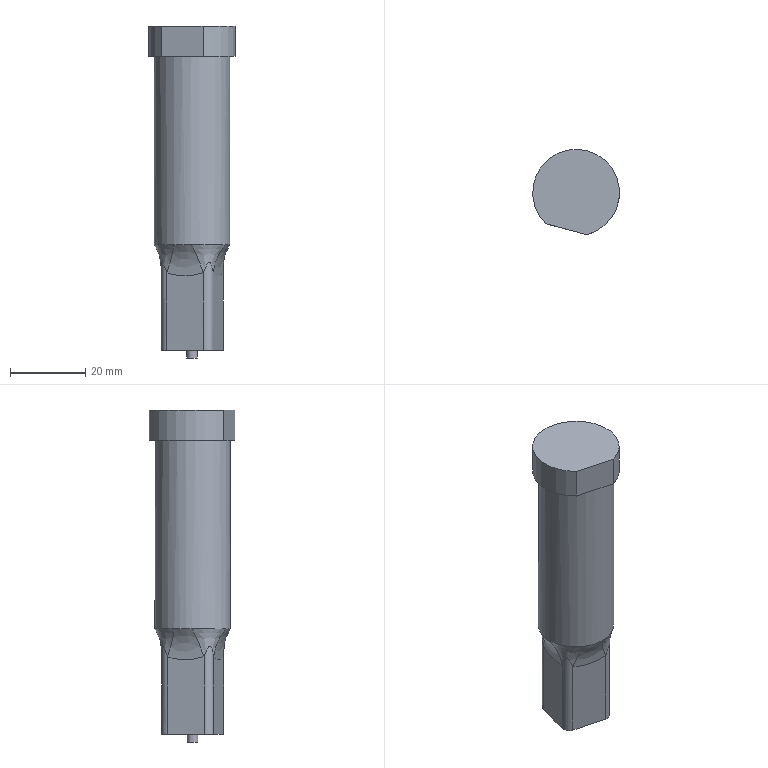Part | NX | features solid 2 | 1 solid | 24 faces | box 23 x 22.629 x 88 mm | volume 24741 mm3 | plane 9 | spline 8 | cylinder 7 | commonest cylinder face diameters 4.15 x4 2.8 x1 20 x1 23 x1
STEP:
#1=CARTESIAN_POINT('',(1379.695,-27.912,20.));
#2=VERTEX_POINT('',#1);
#3=CARTESIAN_POINT('',(1384.847,-36.837,20.));
#4=VERTEX_POINT('',#3);
#5=CARTESIAN_POINT('',(1389.693,-28.089,20.));
#6=DIRECTION('',(0.,0.,1.));
#7=DIRECTION('',(1.,0.,0.));
#8=AXIS2_PLACEMENT_3D('',#5,#6,#7);
#9=CIRCLE('',#8,10.);
#10=EDGE_CURVE('',#2,#4,#9,.T.);
#11=ORIENTED_EDGE('',*,*,#10,.T.);
#12=CARTESIAN_POINT('',(1389.516,-38.088,20.));
#13=VERTEX_POINT('',#12);
#14=CARTESIAN_POINT('',(1389.693,-28.089,20.));
#15=DIRECTION('',(0.,0.,1.));
#16=DIRECTION('',(1.,0.,0.));
#17=AXIS2_PLACEMENT_3D('',#14,#15,#16);
#18=CIRCLE('',#17,10.);
#19=EDGE_CURVE('',#4,#13,#18,.T.);
#20=ORIENTED_EDGE('',*,*,#19,.T.);
#21=CARTESIAN_POINT('',(1398.441,-32.935,20.));
#22=VERTEX_POINT('',#21);
#23=CARTESIAN_POINT('',(1389.693,-28.089,20.));
#24=DIRECTION('',(0.,0.,1.));
#25=DIRECTION('',(1.,0.,0.));
#26=AXIS2_PLACEMENT_3D('',#23,#24,#25);
#27=CIRCLE('',#26,10.);
#28=EDGE_CURVE('',#13,#22,#27,.T.);
#29=ORIENTED_EDGE('',*,*,#28,.T.);
#30=CARTESIAN_POINT('',(1399.692,-28.266,20.));
#31=VERTEX_POINT('',#30);
#32=CARTESIAN_POINT('',(1389.693,-28.089,20.));
#33=DIRECTION('',(0.,0.,1.));
#34=DIRECTION('',(1.,0.,0.));
#35=AXIS2_PLACEMENT_3D('',#32,#33,#34);
#36=CIRCLE('',#35,10.);
#37=EDGE_CURVE('',#22,#31,#36,.T.);
#38=ORIENTED_EDGE('',*,*,#37,.T.);
#39=CARTESIAN_POINT('',(1394.539,-19.342,20.));
#40=VERTEX_POINT('',#39);
#41=CARTESIAN_POINT('',(1389.693,-28.089,20.));
#42=DIRECTION('',(0.,0.,1.));
#43=DIRECTION('',(1.,0.,0.));
#44=AXIS2_PLACEMENT_3D('',#41,#42,#43);
#45=CIRCLE('',#44,10.);
#46=EDGE_CURVE('',#31,#40,#45,.T.);
#47=ORIENTED_EDGE('',*,*,#46,.T.);
#48=CARTESIAN_POINT('',(1389.87,-18.091,20.));
#49=VERTEX_POINT('',#48);
#50=CARTESIAN_POINT('',(1389.693,-28.089,20.));
#51=DIRECTION('',(0.,0.,1.));
#52=DIRECTION('',(1.,0.,0.));
#53=AXIS2_PLACEMENT_3D('',#50,#51,#52);
#54=CIRCLE('',#53,10.);
#55=EDGE_CURVE('',#40,#49,#54,.T.);
#56=ORIENTED_EDGE('',*,*,#55,.T.);
#57=CARTESIAN_POINT('',(1380.946,-23.243,20.));
#58=VERTEX_POINT('',#57);
#59=CARTESIAN_POINT('',(1389.693,-28.089,20.));
#60=DIRECTION('',(0.,0.,1.));
#61=DIRECTION('',(1.,0.,0.));
#62=AXIS2_PLACEMENT_3D('',#59,#60,#61);
#63=CIRCLE('',#62,10.);
#64=EDGE_CURVE('',#49,#58,#63,.T.);
#65=ORIENTED_EDGE('',*,*,#64,.T.);
#66=CARTESIAN_POINT('',(1389.693,-28.089,20.));
#67=DIRECTION('',(0.,0.,1.));
#68=DIRECTION('',(1.,0.,0.));
#69=AXIS2_PLACEMENT_3D('',#66,#67,#68);
#70=CIRCLE('',#69,10.);
#71=EDGE_CURVE('',#58,#2,#70,.T.);
#72=ORIENTED_EDGE('',*,*,#71,.T.);
#73=EDGE_LOOP('',(#11,#20,#29,#38,#47,#56,#65,#72));
#74=FACE_BOUND('',#73,.T.);
#75=CARTESIAN_POINT('',(1387.105,-37.749,70.));
#76=VERTEX_POINT('',#75);
#77=CARTESIAN_POINT('',(1389.693,-28.089,70.));
#78=DIRECTION('',(0.,0.,1.));
#79=DIRECTION('',(1.,0.,0.));
#80=AXIS2_PLACEMENT_3D('',#77,#78,#79);
#81=CIRCLE('',#80,10.);
#82=EDGE_CURVE('',#76,#76,#81,.F.);
#83=ORIENTED_EDGE('',*,*,#82,.T.);
#84=EDGE_LOOP('',(#83));
#85=FACE_BOUND('',#84,.T.);
#86=CARTESIAN_POINT('',(1389.693,-28.089,-26.));
#87=DIRECTION('',(0.,0.,1.));
#88=DIRECTION('',(1.,0.,0.));
#89=AXIS2_PLACEMENT_3D('',#86,#87,#88);
#90=CYLINDRICAL_SURFACE('',#89,10.);
#91=ADVANCED_FACE('',(#74,#85),#90,.T.);
#92=CARTESIAN_POINT('',(1392.591,-39.218,78.));
#93=VERTEX_POINT('',#92);
#94=CARTESIAN_POINT('',(1381.62,-36.279,78.));
#95=VERTEX_POINT('',#94);
#96=CARTESIAN_POINT('',(1389.693,-28.089,78.));
#97=DIRECTION('',(0.,0.,1.));
#98=DIRECTION('',(1.,0.,0.));
#99=AXIS2_PLACEMENT_3D('',#96,#97,#98);
#100=CIRCLE('',#99,11.5);
#101=EDGE_CURVE('',#93,#95,#100,.T.);
#102=ORIENTED_EDGE('',*,*,#101,.F.);
#103=CARTESIAN_POINT('',(1392.591,-39.218,70.));
#104=VERTEX_POINT('',#103);
#105=CARTESIAN_POINT('',(1392.591,-39.218,78.));
#106=DIRECTION('',(0.,0.,-1.));
#107=VECTOR('',#106,1000.);
#108=LINE('',#105,#107);
#109=EDGE_CURVE('',#104,#93,#108,.F.);
#110=ORIENTED_EDGE('',*,*,#109,.F.);
#111=CARTESIAN_POINT('',(1381.62,-36.279,70.));
#112=VERTEX_POINT('',#111);
#113=CARTESIAN_POINT('',(1389.693,-28.089,70.));
#114=DIRECTION('',(0.,0.,1.));
#115=DIRECTION('',(1.,0.,0.));
#116=AXIS2_PLACEMENT_3D('',#113,#114,#115);
#117=CIRCLE('',#116,11.5);
#118=EDGE_CURVE('',#104,#112,#117,.T.);
#119=ORIENTED_EDGE('',*,*,#118,.T.);
#120=CARTESIAN_POINT('',(1381.62,-36.279,78.));
#121=DIRECTION('',(0.,0.,-1.));
#122=VECTOR('',#121,1000.);
#123=LINE('',#120,#122);
#124=EDGE_CURVE('',#95,#112,#123,.T.);
#125=ORIENTED_EDGE('',*,*,#124,.F.);
#126=EDGE_LOOP('',(#102,#110,#119,#125));
#127=FACE_BOUND('',#126,.T.);
#128=CARTESIAN_POINT('',(1389.693,-28.089,78.));
#129=DIRECTION('',(0.,0.,-1.));
#130=DIRECTION('',(-1.,0.,0.));
#131=AXIS2_PLACEMENT_3D('',#128,#129,#130);
#132=CYLINDRICAL_SURFACE('',#131,11.5);
#133=ADVANCED_FACE('',(#127),#132,.T.);
#134=ORIENTED_EDGE('',*,*,#118,.F.);
#135=CARTESIAN_POINT('',(1387.105,-37.749,70.));
#136=DIRECTION('',(-0.9659,0.2588,0.));
#137=VECTOR('',#136,1000.);
#138=LINE('',#135,#137);
#139=EDGE_CURVE('',#104,#76,#138,.T.);
#140=ORIENTED_EDGE('',*,*,#139,.T.);
#141=ORIENTED_EDGE('',*,*,#82,.F.);
#142=CARTESIAN_POINT('',(1387.105,-37.749,70.));
#143=DIRECTION('',(-0.9659,0.2588,0.));
#144=VECTOR('',#143,1000.);
#145=LINE('',#142,#144);
#146=EDGE_CURVE('',#76,#112,#145,.T.);
#147=ORIENTED_EDGE('',*,*,#146,.T.);
#148=EDGE_LOOP('',(#134,#140,#141,#147));
#149=FACE_BOUND('',#148,.T.);
#150=CARTESIAN_POINT('',(1389.693,-28.089,70.));
#151=DIRECTION('',(0.,0.,1.));
#152=DIRECTION('',(1.,0.,0.));
#153=AXIS2_PLACEMENT_3D('',#150,#151,#152);
#154=PLANE('',#153);
#155=ADVANCED_FACE('',(#149),#154,.F.);
#156=ORIENTED_EDGE('',*,*,#101,.T.);
#157=CARTESIAN_POINT('',(2030.826,-210.233,78.));
#158=DIRECTION('',(0.9659,-0.2588,0.));
#159=VECTOR('',#158,1000.);
#160=LINE('',#157,#159);
#161=EDGE_CURVE('',#93,#95,#160,.F.);
#162=ORIENTED_EDGE('',*,*,#161,.F.);
#163=EDGE_LOOP('',(#156,#162));
#164=FACE_BOUND('',#163,.T.);
#165=CARTESIAN_POINT('',(2087.158,-0.000000688,78.));
#166=DIRECTION('',(0.,0.,-1.));
#167=DIRECTION('',(1.,0.,0.));
#168=AXIS2_PLACEMENT_3D('',#165,#166,#167);
#169=PLANE('',#168);
#170=ADVANCED_FACE('',(#164),#169,.F.);
#171=CARTESIAN_POINT('',(1392.692,-36.217,12.6));
#172=VERTEX_POINT('',#171);
#173=CARTESIAN_POINT('',(1392.692,-36.217,-8.));
#174=VERTEX_POINT('',#173);
#175=CARTESIAN_POINT('',(1392.692,-36.217,82.));
#176=DIRECTION('',(0.,0.,1.));
#177=VECTOR('',#176,1000.);
#178=LINE('',#175,#177);
#179=EDGE_CURVE('',#172,#174,#178,.F.);
#180=ORIENTED_EDGE('',*,*,#179,.F.);
#181=CARTESIAN_POINT('',(1383.033,-33.629,12.6));
#182=VERTEX_POINT('',#181);
#183=CARTESIAN_POINT('',(1392.692,-36.217,12.6));
#184=CARTESIAN_POINT('',(1391.934,-36.014,12.326));
#185=CARTESIAN_POINT('',(1390.301,-35.577,11.91));
#186=CARTESIAN_POINT('',(1387.857,-34.922,11.722));
#187=CARTESIAN_POINT('',(1385.431,-34.272,11.909));
#188=CARTESIAN_POINT('',(1383.791,-33.832,12.326));
#189=CARTESIAN_POINT('',(1383.033,-33.629,12.6));
#190=B_SPLINE_CURVE_WITH_KNOTS('',3,(#183,#184,#185,#186,#187,#188,#189),.UNSPECIFIED.,.F.,.F.,(4,1,1,1,4),(0.,0.25,0.5,0.75,1.),.UNSPECIFIED.);
#191=EDGE_CURVE('',#172,#182,#190,.T.);
#192=ORIENTED_EDGE('',*,*,#191,.T.);
#193=CARTESIAN_POINT('',(1383.033,-33.629,-8.));
#194=VERTEX_POINT('',#193);
#195=CARTESIAN_POINT('',(1383.033,-33.629,82.));
#196=DIRECTION('',(0.,0.,-1.));
#197=VECTOR('',#196,1000.);
#198=LINE('',#195,#197);
#199=EDGE_CURVE('',#182,#194,#198,.T.);
#200=ORIENTED_EDGE('',*,*,#199,.T.);
#201=CARTESIAN_POINT('',(1392.692,-36.217,-8.));
#202=DIRECTION('',(0.9659,-0.2588,0.));
#203=VECTOR('',#202,1000.);
#204=LINE('',#201,#203);
#205=EDGE_CURVE('',#194,#174,#204,.T.);
#206=ORIENTED_EDGE('',*,*,#205,.T.);
#207=EDGE_LOOP('',(#180,#192,#200,#206));
#208=FACE_BOUND('',#207,.T.);
#209=CARTESIAN_POINT('',(1383.033,-33.629,82.));
#210=DIRECTION('',(-0.2588,-0.9659,0.));
#211=DIRECTION('',(-0.9659,0.2588,0.));
#212=AXIS2_PLACEMENT_3D('',#209,#210,#211);
#213=PLANE('',#212);
#214=ADVANCED_FACE('',(#208),#213,.T.);
#215=CARTESIAN_POINT('',(1395.233,-34.75,12.6));
#216=VERTEX_POINT('',#215);
#217=CARTESIAN_POINT('',(1395.233,-34.75,-8.));
#218=VERTEX_POINT('',#217);
#219=CARTESIAN_POINT('',(1395.233,-34.75,82.));
#220=DIRECTION('',(0.,0.,-1.));
#221=VECTOR('',#220,1000.);
#222=LINE('',#219,#221);
#223=EDGE_CURVE('',#216,#218,#222,.T.);
#224=ORIENTED_EDGE('',*,*,#223,.F.);
#225=CARTESIAN_POINT('',(1395.233,-34.75,12.6));
#226=CARTESIAN_POINT('',(1395.201,-34.872,12.92));
#227=CARTESIAN_POINT('',(1395.123,-35.069,13.441));
#228=CARTESIAN_POINT('',(1395.032,-35.257,13.948));
#229=CARTESIAN_POINT('',(1394.856,-35.505,14.566));
#230=CARTESIAN_POINT('',(1394.785,-35.59,14.77));
#231=CARTESIAN_POINT('',(1394.652,-35.725,15.047));
#232=CARTESIAN_POINT('',(1394.547,-35.82,15.217));
#233=CARTESIAN_POINT('',(1394.279,-36.022,15.464));
#234=CARTESIAN_POINT('',(1393.966,-36.156,15.222));
#235=CARTESIAN_POINT('',(1393.831,-36.2,15.053));
#236=CARTESIAN_POINT('',(1393.646,-36.249,14.774));
#237=CARTESIAN_POINT('',(1393.537,-36.268,14.571));
#238=CARTESIAN_POINT('',(1393.234,-36.297,13.953));
#239=CARTESIAN_POINT('',(1393.024,-36.282,13.444));
#240=CARTESIAN_POINT('',(1392.814,-36.25,12.921));
#241=CARTESIAN_POINT('',(1392.692,-36.217,12.6));
#242=B_SPLINE_CURVE_WITH_KNOTS('',3,(#225,#226,#227,#228,#229,#230,#231,#232,#233,#234,#235,#236,#237,#238,#239,#240,#241),.UNSPECIFIED.,.F.,.F.,(4,1,1,1,1,1,1,1,1,1,1,1,1,1,4),(0.,0.125,0.25,0.3125,0.375,0.4062,0.4375,0.5,0.5625,0.5938,0.625,0.6875,0.75,0.875,1.),.UNSPECIFIED.);
#243=EDGE_CURVE('',#216,#172,#242,.T.);
#244=ORIENTED_EDGE('',*,*,#243,.T.);
#245=ORIENTED_EDGE('',*,*,#179,.T.);
#246=CARTESIAN_POINT('',(1393.229,-34.213,-8.));
#247=DIRECTION('',(0.,0.,1.));
#248=DIRECTION('',(-1.,0.,0.));
#249=AXIS2_PLACEMENT_3D('',#246,#247,#248);
#250=CIRCLE('',#249,2.075);
#251=EDGE_CURVE('',#174,#218,#250,.T.);
#252=ORIENTED_EDGE('',*,*,#251,.T.);
#253=EDGE_LOOP('',(#224,#244,#245,#252));
#254=FACE_BOUND('',#253,.T.);
#255=CARTESIAN_POINT('',(1393.229,-34.213,82.));
#256=DIRECTION('',(0.,0.,-1.));
#257=DIRECTION('',(-1.,0.,0.));
#258=AXIS2_PLACEMENT_3D('',#255,#256,#257);
#259=CYLINDRICAL_SURFACE('',#258,2.075);
#260=ADVANCED_FACE('',(#254),#259,.T.);
#261=CARTESIAN_POINT('',(1397.821,-25.091,12.6));
#262=VERTEX_POINT('',#261);
#263=CARTESIAN_POINT('',(1397.821,-25.091,-8.));
#264=VERTEX_POINT('',#263);
#265=CARTESIAN_POINT('',(1397.821,-25.091,82.));
#266=DIRECTION('',(0.,0.,1.));
#267=VECTOR('',#266,1000.);
#268=LINE('',#265,#267);
#269=EDGE_CURVE('',#262,#264,#268,.F.);
#270=ORIENTED_EDGE('',*,*,#269,.F.);
#271=CARTESIAN_POINT('',(1397.821,-25.091,12.6));
#272=CARTESIAN_POINT('',(1397.618,-25.848,12.326));
#273=CARTESIAN_POINT('',(1397.181,-27.482,11.91));
#274=CARTESIAN_POINT('',(1396.526,-29.925,11.722));
#275=CARTESIAN_POINT('',(1395.876,-32.352,11.909));
#276=CARTESIAN_POINT('',(1395.437,-33.991,12.326));
#277=CARTESIAN_POINT('',(1395.233,-34.75,12.6));
#278=B_SPLINE_CURVE_WITH_KNOTS('',3,(#271,#272,#273,#274,#275,#276,#277),.UNSPECIFIED.,.F.,.F.,(4,1,1,1,4),(0.,0.25,0.5,0.75,1.),.UNSPECIFIED.);
#279=EDGE_CURVE('',#262,#216,#278,.T.);
#280=ORIENTED_EDGE('',*,*,#279,.T.);
#281=ORIENTED_EDGE('',*,*,#223,.T.);
#282=CARTESIAN_POINT('',(1395.233,-34.75,-8.));
#283=DIRECTION('',(0.2588,0.9659,0.));
#284=VECTOR('',#283,1000.);
#285=LINE('',#282,#284);
#286=EDGE_CURVE('',#218,#264,#285,.T.);
#287=ORIENTED_EDGE('',*,*,#286,.T.);
#288=EDGE_LOOP('',(#270,#280,#281,#287));
#289=FACE_BOUND('',#288,.T.);
#290=CARTESIAN_POINT('',(1395.233,-34.75,82.));
#291=DIRECTION('',(0.9659,-0.2588,0.));
#292=DIRECTION('',(-0.2588,-0.9659,0.));
#293=AXIS2_PLACEMENT_3D('',#290,#291,#292);
#294=PLANE('',#293);
#295=ADVANCED_FACE('',(#289),#294,.T.);
#296=CARTESIAN_POINT('',(1396.354,-22.55,12.6));
#297=VERTEX_POINT('',#296);
#298=CARTESIAN_POINT('',(1396.354,-22.55,-8.));
#299=VERTEX_POINT('',#298);
#300=CARTESIAN_POINT('',(1396.354,-22.55,82.));
#301=DIRECTION('',(0.,0.,-1.));
#302=VECTOR('',#301,1000.);
#303=LINE('',#300,#302);
#304=EDGE_CURVE('',#297,#299,#303,.T.);
#305=ORIENTED_EDGE('',*,*,#304,.F.);
#306=CARTESIAN_POINT('',(1396.354,-22.55,12.6));
#307=CARTESIAN_POINT('',(1396.476,-22.582,12.92));
#308=CARTESIAN_POINT('',(1396.673,-22.659,13.441));
#309=CARTESIAN_POINT('',(1396.861,-22.751,13.948));
#310=CARTESIAN_POINT('',(1397.109,-22.927,14.566));
#311=CARTESIAN_POINT('',(1397.194,-22.998,14.77));
#312=CARTESIAN_POINT('',(1397.329,-23.131,15.047));
#313=CARTESIAN_POINT('',(1397.424,-23.236,15.217));
#314=CARTESIAN_POINT('',(1397.626,-23.504,15.464));
#315=CARTESIAN_POINT('',(1397.76,-23.817,15.222));
#316=CARTESIAN_POINT('',(1397.804,-23.952,15.053));
#317=CARTESIAN_POINT('',(1397.853,-24.137,14.774));
#318=CARTESIAN_POINT('',(1397.872,-24.246,14.571));
#319=CARTESIAN_POINT('',(1397.901,-24.549,13.953));
#320=CARTESIAN_POINT('',(1397.886,-24.759,13.444));
#321=CARTESIAN_POINT('',(1397.854,-24.969,12.921));
#322=CARTESIAN_POINT('',(1397.821,-25.091,12.6));
#323=B_SPLINE_CURVE_WITH_KNOTS('',3,(#306,#307,#308,#309,#310,#311,#312,#313,#314,#315,#316,#317,#318,#319,#320,#321,#322),.UNSPECIFIED.,.F.,.F.,(4,1,1,1,1,1,1,1,1,1,1,1,1,1,4),(0.,0.125,0.25,0.3125,0.375,0.4062,0.4375,0.5,0.5625,0.5938,0.625,0.6875,0.75,0.875,1.),.UNSPECIFIED.);
#324=EDGE_CURVE('',#297,#262,#323,.T.);
#325=ORIENTED_EDGE('',*,*,#324,.T.);
#326=ORIENTED_EDGE('',*,*,#269,.T.);
#327=CARTESIAN_POINT('',(1395.817,-24.554,-8.));
#328=DIRECTION('',(0.,0.,1.));
#329=DIRECTION('',(-1.,0.,0.));
#330=AXIS2_PLACEMENT_3D('',#327,#328,#329);
#331=CIRCLE('',#330,2.075);
#332=EDGE_CURVE('',#264,#299,#331,.T.);
#333=ORIENTED_EDGE('',*,*,#332,.T.);
#334=EDGE_LOOP('',(#305,#325,#326,#333));
#335=FACE_BOUND('',#334,.T.);
#336=CARTESIAN_POINT('',(1395.817,-24.554,82.));
#337=DIRECTION('',(0.,0.,-1.));
#338=DIRECTION('',(-1.,0.,0.));
#339=AXIS2_PLACEMENT_3D('',#336,#337,#338);
#340=CYLINDRICAL_SURFACE('',#339,2.075);
#341=ADVANCED_FACE('',(#335),#340,.T.);
#342=CARTESIAN_POINT('',(1386.695,-19.961,12.6));
#343=VERTEX_POINT('',#342);
#344=CARTESIAN_POINT('',(1386.695,-19.961,-8.));
#345=VERTEX_POINT('',#344);
#346=CARTESIAN_POINT('',(1386.695,-19.961,82.));
#347=DIRECTION('',(0.,0.,1.));
#348=VECTOR('',#347,1000.);
#349=LINE('',#346,#348);
#350=EDGE_CURVE('',#343,#345,#349,.F.);
#351=ORIENTED_EDGE('',*,*,#350,.F.);
#352=CARTESIAN_POINT('',(1386.695,-19.961,12.6));
#353=CARTESIAN_POINT('',(1387.452,-20.164,12.326));
#354=CARTESIAN_POINT('',(1389.086,-20.602,11.91));
#355=CARTESIAN_POINT('',(1391.529,-21.257,11.722));
#356=CARTESIAN_POINT('',(1393.956,-21.907,11.909));
#357=CARTESIAN_POINT('',(1395.596,-22.346,12.326));
#358=CARTESIAN_POINT('',(1396.354,-22.55,12.6));
#359=B_SPLINE_CURVE_WITH_KNOTS('',3,(#352,#353,#354,#355,#356,#357,#358),.UNSPECIFIED.,.F.,.F.,(4,1,1,1,4),(0.,0.25,0.5,0.75,1.),.UNSPECIFIED.);
#360=EDGE_CURVE('',#343,#297,#359,.T.);
#361=ORIENTED_EDGE('',*,*,#360,.T.);
#362=ORIENTED_EDGE('',*,*,#304,.T.);
#363=CARTESIAN_POINT('',(1396.354,-22.55,-8.));
#364=DIRECTION('',(-0.9659,0.2588,0.));
#365=VECTOR('',#364,1000.);
#366=LINE('',#363,#365);
#367=EDGE_CURVE('',#299,#345,#366,.T.);
#368=ORIENTED_EDGE('',*,*,#367,.T.);
#369=EDGE_LOOP('',(#351,#361,#362,#368));
#370=FACE_BOUND('',#369,.T.);
#371=CARTESIAN_POINT('',(1396.354,-22.55,82.));
#372=DIRECTION('',(0.2588,0.9659,0.));
#373=DIRECTION('',(0.9659,-0.2588,0.));
#374=AXIS2_PLACEMENT_3D('',#371,#372,#373);
#375=PLANE('',#374);
#376=ADVANCED_FACE('',(#370),#375,.T.);
#377=CARTESIAN_POINT('',(1384.154,-21.429,12.6));
#378=VERTEX_POINT('',#377);
#379=CARTESIAN_POINT('',(1384.154,-21.429,-8.));
#380=VERTEX_POINT('',#379);
#381=CARTESIAN_POINT('',(1384.154,-21.429,82.));
#382=DIRECTION('',(0.,0.,-1.));
#383=VECTOR('',#382,1000.);
#384=LINE('',#381,#383);
#385=EDGE_CURVE('',#378,#380,#384,.T.);
#386=ORIENTED_EDGE('',*,*,#385,.F.);
#387=CARTESIAN_POINT('',(1384.154,-21.429,12.6));
#388=CARTESIAN_POINT('',(1384.186,-21.307,12.92));
#389=CARTESIAN_POINT('',(1384.263,-21.11,13.441));
#390=CARTESIAN_POINT('',(1384.355,-20.921,13.948));
#391=CARTESIAN_POINT('',(1384.531,-20.674,14.566));
#392=CARTESIAN_POINT('',(1384.602,-20.589,14.77));
#393=CARTESIAN_POINT('',(1384.735,-20.454,15.047));
#394=CARTESIAN_POINT('',(1384.84,-20.359,15.217));
#395=CARTESIAN_POINT('',(1385.108,-20.157,15.464));
#396=CARTESIAN_POINT('',(1385.421,-20.023,15.222));
#397=CARTESIAN_POINT('',(1385.556,-19.979,15.053));
#398=CARTESIAN_POINT('',(1385.741,-19.93,14.774));
#399=CARTESIAN_POINT('',(1385.85,-19.911,14.571));
#400=CARTESIAN_POINT('',(1386.153,-19.882,13.953));
#401=CARTESIAN_POINT('',(1386.363,-19.897,13.444));
#402=CARTESIAN_POINT('',(1386.573,-19.929,12.921));
#403=CARTESIAN_POINT('',(1386.695,-19.961,12.6));
#404=B_SPLINE_CURVE_WITH_KNOTS('',3,(#387,#388,#389,#390,#391,#392,#393,#394,#395,#396,#397,#398,#399,#400,#401,#402,#403),.UNSPECIFIED.,.F.,.F.,(4,1,1,1,1,1,1,1,1,1,1,1,1,1,4),(0.,0.125,0.25,0.3125,0.375,0.4062,0.4375,0.5,0.5625,0.5938,0.625,0.6875,0.75,0.875,1.),.UNSPECIFIED.);
#405=EDGE_CURVE('',#378,#343,#404,.T.);
#406=ORIENTED_EDGE('',*,*,#405,.T.);
#407=ORIENTED_EDGE('',*,*,#350,.T.);
#408=CARTESIAN_POINT('',(1386.158,-21.966,-8.));
#409=DIRECTION('',(0.,0.,1.));
#410=DIRECTION('',(-1.,0.,0.));
#411=AXIS2_PLACEMENT_3D('',#408,#409,#410);
#412=CIRCLE('',#411,2.075);
#413=EDGE_CURVE('',#345,#380,#412,.T.);
#414=ORIENTED_EDGE('',*,*,#413,.T.);
#415=EDGE_LOOP('',(#386,#406,#407,#414));
#416=FACE_BOUND('',#415,.T.);
#417=CARTESIAN_POINT('',(1386.158,-21.966,82.));
#418=DIRECTION('',(0.,0.,-1.));
#419=DIRECTION('',(-1.,0.,0.));
#420=AXIS2_PLACEMENT_3D('',#417,#418,#419);
#421=CYLINDRICAL_SURFACE('',#420,2.075);
#422=ADVANCED_FACE('',(#416),#421,.T.);
#423=CARTESIAN_POINT('',(1381.565,-31.088,12.6));
#424=VERTEX_POINT('',#423);
#425=CARTESIAN_POINT('',(1381.565,-31.088,-8.));
#426=VERTEX_POINT('',#425);
#427=CARTESIAN_POINT('',(1381.565,-31.088,82.));
#428=DIRECTION('',(0.,0.,1.));
#429=VECTOR('',#428,1000.);
#430=LINE('',#427,#429);
#431=EDGE_CURVE('',#424,#426,#430,.F.);
#432=ORIENTED_EDGE('',*,*,#431,.F.);
#433=CARTESIAN_POINT('',(1381.565,-31.088,12.6));
#434=CARTESIAN_POINT('',(1381.768,-30.33,12.326));
#435=CARTESIAN_POINT('',(1382.206,-28.697,11.91));
#436=CARTESIAN_POINT('',(1382.861,-26.253,11.722));
#437=CARTESIAN_POINT('',(1383.511,-23.827,11.909));
#438=CARTESIAN_POINT('',(1383.95,-22.187,12.326));
#439=CARTESIAN_POINT('',(1384.154,-21.429,12.6));
#440=B_SPLINE_CURVE_WITH_KNOTS('',3,(#433,#434,#435,#436,#437,#438,#439),.UNSPECIFIED.,.F.,.F.,(4,1,1,1,4),(0.,0.25,0.5,0.75,1.),.UNSPECIFIED.);
#441=EDGE_CURVE('',#424,#378,#440,.T.);
#442=ORIENTED_EDGE('',*,*,#441,.T.);
#443=ORIENTED_EDGE('',*,*,#385,.T.);
#444=CARTESIAN_POINT('',(1381.565,-31.088,-8.));
#445=DIRECTION('',(-0.2588,-0.9659,0.));
#446=VECTOR('',#445,1000.);
#447=LINE('',#444,#446);
#448=EDGE_CURVE('',#380,#426,#447,.T.);
#449=ORIENTED_EDGE('',*,*,#448,.T.);
#450=EDGE_LOOP('',(#432,#442,#443,#449));
#451=FACE_BOUND('',#450,.T.);
#452=CARTESIAN_POINT('',(1384.154,-21.429,82.));
#453=DIRECTION('',(-0.9659,0.2588,0.));
#454=DIRECTION('',(0.2588,0.9659,0.));
#455=AXIS2_PLACEMENT_3D('',#452,#453,#454);
#456=PLANE('',#455);
#457=ADVANCED_FACE('',(#451),#456,.T.);
#458=ORIENTED_EDGE('',*,*,#199,.F.);
#459=CARTESIAN_POINT('',(1383.033,-33.629,12.6));
#460=CARTESIAN_POINT('',(1382.911,-33.597,12.92));
#461=CARTESIAN_POINT('',(1382.714,-33.519,13.441));
#462=CARTESIAN_POINT('',(1382.526,-33.428,13.948));
#463=CARTESIAN_POINT('',(1382.278,-33.252,14.566));
#464=CARTESIAN_POINT('',(1382.193,-33.181,14.77));
#465=CARTESIAN_POINT('',(1382.058,-33.048,15.047));
#466=CARTESIAN_POINT('',(1381.963,-32.943,15.217));
#467=CARTESIAN_POINT('',(1381.761,-32.675,15.464));
#468=CARTESIAN_POINT('',(1381.627,-32.362,15.222));
#469=CARTESIAN_POINT('',(1381.583,-32.227,15.053));
#470=CARTESIAN_POINT('',(1381.534,-32.041,14.773));
#471=CARTESIAN_POINT('',(1381.515,-31.934,14.574));
#472=CARTESIAN_POINT('',(1381.493,-31.699,14.094));
#473=CARTESIAN_POINT('',(1381.495,-31.57,13.797));
#474=CARTESIAN_POINT('',(1381.504,-31.389,13.37));
#475=CARTESIAN_POINT('',(1381.531,-31.215,12.933));
#476=CARTESIAN_POINT('',(1381.565,-31.088,12.6));
#477=B_SPLINE_CURVE_WITH_KNOTS('',3,(#459,#460,#461,#462,#463,#464,#465,#466,#467,#468,#469,#470,#471,#472,#473,#474,#475,#476),.UNSPECIFIED.,.F.,.F.,(4,1,1,1,1,1,1,1,1,1,1,1,1,1,1,4),(0.,0.125,0.25,0.3125,0.375,0.4062,0.4375,0.5,0.5625,0.5938,0.625,0.6875,0.75,0.8125,0.875,1.),.UNSPECIFIED.);
#478=EDGE_CURVE('',#182,#424,#477,.T.);
#479=ORIENTED_EDGE('',*,*,#478,.T.);
#480=ORIENTED_EDGE('',*,*,#431,.T.);
#481=CARTESIAN_POINT('',(1383.57,-31.625,-8.));
#482=DIRECTION('',(0.,0.,1.));
#483=DIRECTION('',(-1.,0.,0.));
#484=AXIS2_PLACEMENT_3D('',#481,#482,#483);
#485=CIRCLE('',#484,2.075);
#486=EDGE_CURVE('',#426,#194,#485,.T.);
#487=ORIENTED_EDGE('',*,*,#486,.T.);
#488=EDGE_LOOP('',(#458,#479,#480,#487));
#489=FACE_BOUND('',#488,.T.);
#490=CARTESIAN_POINT('',(1383.57,-31.625,82.));
#491=DIRECTION('',(0.,0.,-1.));
#492=DIRECTION('',(-1.,0.,0.));
#493=AXIS2_PLACEMENT_3D('',#490,#491,#492);
#494=CYLINDRICAL_SURFACE('',#493,2.075);
#495=ADVANCED_FACE('',(#489),#494,.T.);
#496=CARTESIAN_POINT('',(1388.293,-28.089,-8.));
#497=VERTEX_POINT('',#496);
#498=CARTESIAN_POINT('',(1389.693,-28.089,-8.));
#499=DIRECTION('',(0.,0.,-1.));
#500=DIRECTION('',(-1.,0.,0.));
#501=AXIS2_PLACEMENT_3D('',#498,#499,#500);
#502=CIRCLE('',#501,1.4);
#503=EDGE_CURVE('',#497,#497,#502,.T.);
#504=ORIENTED_EDGE('',*,*,#503,.F.);
#505=EDGE_LOOP('',(#504));
#506=FACE_BOUND('',#505,.T.);
#507=ORIENTED_EDGE('',*,*,#205,.F.);
#508=ORIENTED_EDGE('',*,*,#486,.F.);
#509=ORIENTED_EDGE('',*,*,#448,.F.);
#510=ORIENTED_EDGE('',*,*,#413,.F.);
#511=ORIENTED_EDGE('',*,*,#367,.F.);
#512=ORIENTED_EDGE('',*,*,#332,.F.);
#513=ORIENTED_EDGE('',*,*,#286,.F.);
#514=ORIENTED_EDGE('',*,*,#251,.F.);
#515=EDGE_LOOP('',(#507,#508,#509,#510,#511,#512,#513,#514));
#516=FACE_BOUND('',#515,.T.);
#517=CARTESIAN_POINT('',(1393.229,-34.213,-8.));
#518=DIRECTION('',(0.,0.,-1.));
#519=DIRECTION('',(-1.,0.,0.));
#520=AXIS2_PLACEMENT_3D('',#517,#518,#519);
#521=PLANE('',#520);
#522=ADVANCED_FACE('',(#506,#516),#521,.T.);
#523=CARTESIAN_POINT('',(1407.79,-38.115,12.6));
#524=DIRECTION('',(-0.2444,-0.912,0.3296));
#525=DIRECTION('',(0.,-0.3399,-0.9405));
#526=AXIS2_PLACEMENT_3D('',#523,#524,#525);
#527=CIRCLE('',#526,13.);
#528=EDGE_CURVE('',#22,#216,#527,.T.);
#529=ORIENTED_EDGE('',*,*,#528,.F.);
#530=ORIENTED_EDGE('',*,*,#28,.F.);
#531=CARTESIAN_POINT('',(1389.327,-48.774,12.6));
#532=DIRECTION('',(-0.912,0.2444,-0.3296));
#533=DIRECTION('',(-0.3399,0.,0.9405));
#534=AXIS2_PLACEMENT_3D('',#531,#532,#533);
#535=CIRCLE('',#534,13.);
#536=EDGE_CURVE('',#172,#13,#535,.F.);
#537=ORIENTED_EDGE('',*,*,#536,.F.);
#538=ORIENTED_EDGE('',*,*,#243,.F.);
#539=EDGE_LOOP('',(#529,#530,#537,#538));
#540=FACE_BOUND('',#539,.T.);
#541=CARTESIAN_POINT('',(1389.516,-38.088,20.));
#542=CARTESIAN_POINT('',(1391.304,-35.845,16.716));
#543=CARTESIAN_POINT('',(1392.692,-36.217,12.6));
#544=CARTESIAN_POINT('',(1390.414,-38.104,20.));
#545=CARTESIAN_POINT('',(1391.686,-36.134,16.914));
#546=CARTESIAN_POINT('',(1392.946,-36.286,13.268));
#547=CARTESIAN_POINT('',(1392.181,-37.9,20.));
#548=CARTESIAN_POINT('',(1392.657,-36.526,17.419));
#549=CARTESIAN_POINT('',(1393.482,-36.327,14.609));
#550=CARTESIAN_POINT('',(1394.752,-36.864,20.));
#551=CARTESIAN_POINT('',(1394.351,-36.164,17.931));
#552=CARTESIAN_POINT('',(1394.294,-36.062,15.743));
#553=CARTESIAN_POINT('',(1396.939,-35.158,20.));
#554=CARTESIAN_POINT('',(1395.516,-34.881,17.422));
#555=CARTESIAN_POINT('',(1394.931,-35.492,14.617));
#556=CARTESIAN_POINT('',(1398.004,-33.723,20.));
#557=CARTESIAN_POINT('',(1395.665,-33.839,16.915));
#558=CARTESIAN_POINT('',(1395.165,-35.005,13.27));
#559=CARTESIAN_POINT('',(1398.441,-32.935,20.));
#560=CARTESIAN_POINT('',(1395.605,-33.362,16.716));
#561=CARTESIAN_POINT('',(1395.233,-34.75,12.6));
#562=(BOUNDED_SURFACE()B_SPLINE_SURFACE(3,2,((#541,#542,#543),(#544,#545,#546),(#547,#548,#549),(#550,#551,#552),(#553,#554,#555),(#556,#557,#558),(#559,#560,#561)),.UNSPECIFIED.,.F.,.F.,.F.)B_SPLINE_SURFACE_WITH_KNOTS((4,1,1,1,4),(3,3),(0.03889,0.04496,0.05103,0.05711,0.06318),(0.,1.),.UNSPECIFIED.)GEOMETRIC_REPRESENTATION_ITEM()RATIONAL_B_SPLINE_SURFACE(((1.,0.9481,1.),(1.,0.9592,1.),(1.,0.9768,1.),(1.,0.9868,1.),(1.,0.9768,1.),(1.,0.9592,1.),(1.,0.9481,1.)))REPRESENTATION_ITEM('')SURFACE());
#563=ADVANCED_FACE('',(#540),#562,.F.);
#564=ORIENTED_EDGE('',*,*,#536,.T.);
#565=ORIENTED_EDGE('',*,*,#19,.F.);
#566=CARTESIAN_POINT('',(1379.668,-46.186,12.6));
#567=DIRECTION('',(-0.912,0.2444,0.3296));
#568=DIRECTION('',(0.3399,0.,0.9405));
#569=AXIS2_PLACEMENT_3D('',#566,#567,#568);
#570=CIRCLE('',#569,13.);
#571=EDGE_CURVE('',#182,#4,#570,.F.);
#572=ORIENTED_EDGE('',*,*,#571,.F.);
#573=ORIENTED_EDGE('',*,*,#191,.F.);
#574=EDGE_LOOP('',(#564,#565,#572,#573));
#575=FACE_BOUND('',#574,.T.);
#576=CARTESIAN_POINT('',(1384.847,-36.837,20.));
#577=CARTESIAN_POINT('',(1384.421,-34.001,16.716));
#578=CARTESIAN_POINT('',(1383.033,-33.629,12.6));
#579=CARTESIAN_POINT('',(1386.158,-37.563,20.));
#580=CARTESIAN_POINT('',(1386.609,-34.588,16.282));
#581=CARTESIAN_POINT('',(1386.118,-34.456,11.485));
#582=CARTESIAN_POINT('',(1388.018,-38.061,20.));
#583=CARTESIAN_POINT('',(1389.114,-35.259,16.281));
#584=CARTESIAN_POINT('',(1389.605,-35.39,11.484));
#585=CARTESIAN_POINT('',(1389.516,-38.088,20.));
#586=CARTESIAN_POINT('',(1391.304,-35.845,16.716));
#587=CARTESIAN_POINT('',(1392.692,-36.217,12.6));
#588=(BOUNDED_SURFACE()B_SPLINE_SURFACE(3,2,((#576,#577,#578),(#579,#580,#581),(#582,#583,#584),(#585,#586,#587)),.UNSPECIFIED.,.F.,.F.,.F.)B_SPLINE_SURFACE_WITH_KNOTS((4,4),(3,3),(0.01026,0.02041),(0.,1.),.PIECEWISE_BEZIER_KNOTS.)GEOMETRIC_REPRESENTATION_ITEM()RATIONAL_B_SPLINE_SURFACE(((1.,0.9481,1.),(1.,0.9408,1.),(1.,0.9408,1.),(1.,0.9481,1.)))REPRESENTATION_ITEM('')SURFACE());
#589=ADVANCED_FACE('',(#575),#588,.F.);
#590=ORIENTED_EDGE('',*,*,#528,.T.);
#591=ORIENTED_EDGE('',*,*,#279,.F.);
#592=CARTESIAN_POINT('',(1410.378,-28.456,12.6));
#593=DIRECTION('',(-0.2444,-0.912,-0.3296));
#594=DIRECTION('',(0.,0.3399,-0.9405));
#595=AXIS2_PLACEMENT_3D('',#592,#593,#594);
#596=CIRCLE('',#595,13.);
#597=EDGE_CURVE('',#31,#262,#596,.T.);
#598=ORIENTED_EDGE('',*,*,#597,.F.);
#599=ORIENTED_EDGE('',*,*,#37,.F.);
#600=EDGE_LOOP('',(#590,#591,#598,#599));
#601=FACE_BOUND('',#600,.T.);
#602=CARTESIAN_POINT('',(1398.441,-32.935,20.));
#603=CARTESIAN_POINT('',(1395.605,-33.362,16.716));
#604=CARTESIAN_POINT('',(1395.233,-34.75,12.6));
#605=CARTESIAN_POINT('',(1399.167,-31.625,20.));
#606=CARTESIAN_POINT('',(1396.192,-31.173,16.282));
#607=CARTESIAN_POINT('',(1396.06,-31.664,11.485));
#608=CARTESIAN_POINT('',(1399.665,-29.765,20.));
#609=CARTESIAN_POINT('',(1396.863,-28.669,16.281));
#610=CARTESIAN_POINT('',(1396.994,-28.178,11.484));
#611=CARTESIAN_POINT('',(1399.692,-28.266,20.));
#612=CARTESIAN_POINT('',(1397.45,-26.479,16.716));
#613=CARTESIAN_POINT('',(1397.821,-25.091,12.6));
#614=(BOUNDED_SURFACE()B_SPLINE_SURFACE(3,2,((#602,#603,#604),(#605,#606,#607),(#608,#609,#610),(#611,#612,#613)),.UNSPECIFIED.,.F.,.F.,.F.)B_SPLINE_SURFACE_WITH_KNOTS((4,4),(3,3),(0.01026,0.02041),(0.,1.),.PIECEWISE_BEZIER_KNOTS.)GEOMETRIC_REPRESENTATION_ITEM()RATIONAL_B_SPLINE_SURFACE(((1.,0.9481,1.),(1.,0.9408,1.),(1.,0.9408,1.),(1.,0.9481,1.)))REPRESENTATION_ITEM('')SURFACE());
#615=ADVANCED_FACE('',(#601),#614,.F.);
#616=ORIENTED_EDGE('',*,*,#571,.T.);
#617=ORIENTED_EDGE('',*,*,#10,.F.);
#618=CARTESIAN_POINT('',(1369.008,-27.723,12.6));
#619=DIRECTION('',(0.2444,0.912,-0.3296));
#620=DIRECTION('',(0.,0.3399,0.9405));
#621=AXIS2_PLACEMENT_3D('',#618,#619,#620);
#622=CIRCLE('',#621,13.);
#623=EDGE_CURVE('',#424,#2,#622,.F.);
#624=ORIENTED_EDGE('',*,*,#623,.F.);
#625=ORIENTED_EDGE('',*,*,#478,.F.);
#626=EDGE_LOOP('',(#616,#617,#624,#625));
#627=FACE_BOUND('',#626,.T.);
#628=CARTESIAN_POINT('',(1379.695,-27.912,20.));
#629=CARTESIAN_POINT('',(1381.937,-29.7,16.716));
#630=CARTESIAN_POINT('',(1381.565,-31.088,12.6));
#631=CARTESIAN_POINT('',(1379.679,-28.81,20.));
#632=CARTESIAN_POINT('',(1381.648,-30.082,16.914));
#633=CARTESIAN_POINT('',(1381.497,-31.342,13.268));
#634=CARTESIAN_POINT('',(1379.883,-30.577,20.));
#635=CARTESIAN_POINT('',(1381.256,-31.053,17.419));
#636=CARTESIAN_POINT('',(1381.456,-31.878,14.609));
#637=CARTESIAN_POINT('',(1380.918,-33.148,20.));
#638=CARTESIAN_POINT('',(1381.618,-32.747,17.931));
#639=CARTESIAN_POINT('',(1381.721,-32.69,15.743));
#640=CARTESIAN_POINT('',(1382.625,-35.334,20.));
#641=CARTESIAN_POINT('',(1382.902,-33.912,17.422));
#642=CARTESIAN_POINT('',(1382.291,-33.327,14.617));
#643=CARTESIAN_POINT('',(1384.06,-36.4,20.));
#644=CARTESIAN_POINT('',(1383.943,-34.06,16.915));
#645=CARTESIAN_POINT('',(1382.777,-33.561,13.27));
#646=CARTESIAN_POINT('',(1384.847,-36.837,20.));
#647=CARTESIAN_POINT('',(1384.421,-34.001,16.716));
#648=CARTESIAN_POINT('',(1383.033,-33.629,12.6));
#649=(BOUNDED_SURFACE()B_SPLINE_SURFACE(3,2,((#628,#629,#630),(#631,#632,#633),(#634,#635,#636),(#637,#638,#639),(#640,#641,#642),(#643,#644,#645),(#646,#647,#648)),.UNSPECIFIED.,.F.,.F.,.F.)B_SPLINE_SURFACE_WITH_KNOTS((4,1,1,1,4),(3,3),(0.03889,0.04496,0.05103,0.05711,0.06318),(0.,1.),.UNSPECIFIED.)GEOMETRIC_REPRESENTATION_ITEM()RATIONAL_B_SPLINE_SURFACE(((1.,0.9481,1.),(1.,0.9592,1.),(1.,0.9768,1.),(1.,0.9868,1.),(1.,0.9768,1.),(1.,0.9592,1.),(1.,0.9481,1.)))REPRESENTATION_ITEM('')SURFACE());
#650=ADVANCED_FACE('',(#627),#649,.F.);
#651=ORIENTED_EDGE('',*,*,#597,.T.);
#652=ORIENTED_EDGE('',*,*,#324,.F.);
#653=CARTESIAN_POINT('',(1399.719,-9.992,12.6));
#654=DIRECTION('',(0.912,-0.2444,0.3296));
#655=DIRECTION('',(0.3399,0.,-0.9405));
#656=AXIS2_PLACEMENT_3D('',#653,#654,#655);
#657=CIRCLE('',#656,13.);
#658=EDGE_CURVE('',#40,#297,#657,.T.);
#659=ORIENTED_EDGE('',*,*,#658,.F.);
#660=ORIENTED_EDGE('',*,*,#46,.F.);
#661=EDGE_LOOP('',(#651,#652,#659,#660));
#662=FACE_BOUND('',#661,.T.);
#663=CARTESIAN_POINT('',(1399.692,-28.266,20.));
#664=CARTESIAN_POINT('',(1397.45,-26.479,16.716));
#665=CARTESIAN_POINT('',(1397.821,-25.091,12.6));
#666=CARTESIAN_POINT('',(1399.708,-27.369,20.));
#667=CARTESIAN_POINT('',(1397.739,-26.097,16.914));
#668=CARTESIAN_POINT('',(1397.89,-24.836,13.268));
#669=CARTESIAN_POINT('',(1399.504,-25.602,20.));
#670=CARTESIAN_POINT('',(1398.13,-25.126,17.419));
#671=CARTESIAN_POINT('',(1397.931,-24.301,14.609));
#672=CARTESIAN_POINT('',(1398.468,-23.03,20.));
#673=CARTESIAN_POINT('',(1397.769,-23.432,17.931));
#674=CARTESIAN_POINT('',(1397.666,-23.489,15.743));
#675=CARTESIAN_POINT('',(1396.762,-20.844,20.));
#676=CARTESIAN_POINT('',(1396.485,-22.267,17.422));
#677=CARTESIAN_POINT('',(1397.096,-22.852,14.617));
#678=CARTESIAN_POINT('',(1395.327,-19.778,20.));
#679=CARTESIAN_POINT('',(1395.443,-22.118,16.915));
#680=CARTESIAN_POINT('',(1396.609,-22.618,13.27));
#681=CARTESIAN_POINT('',(1394.539,-19.342,20.));
#682=CARTESIAN_POINT('',(1394.966,-22.178,16.716));
#683=CARTESIAN_POINT('',(1396.354,-22.55,12.6));
#684=(BOUNDED_SURFACE()B_SPLINE_SURFACE(3,2,((#663,#664,#665),(#666,#667,#668),(#669,#670,#671),(#672,#673,#674),(#675,#676,#677),(#678,#679,#680),(#681,#682,#683)),.UNSPECIFIED.,.F.,.F.,.F.)B_SPLINE_SURFACE_WITH_KNOTS((4,1,1,1,4),(3,3),(0.03889,0.04496,0.05103,0.05711,0.06318),(0.,1.),.UNSPECIFIED.)GEOMETRIC_REPRESENTATION_ITEM()RATIONAL_B_SPLINE_SURFACE(((1.,0.9481,1.),(1.,0.9592,1.),(1.,0.9768,1.),(1.,0.9868,1.),(1.,0.9768,1.),(1.,0.9592,1.),(1.,0.9481,1.)))REPRESENTATION_ITEM('')SURFACE());
#685=ADVANCED_FACE('',(#662),#684,.F.);
#686=ORIENTED_EDGE('',*,*,#623,.T.);
#687=ORIENTED_EDGE('',*,*,#71,.F.);
#688=CARTESIAN_POINT('',(1371.597,-18.064,12.6));
#689=DIRECTION('',(0.2444,0.912,0.3296));
#690=DIRECTION('',(0.,-0.3399,0.9405));
#691=AXIS2_PLACEMENT_3D('',#688,#689,#690);
#692=CIRCLE('',#691,13.);
#693=EDGE_CURVE('',#378,#58,#692,.F.);
#694=ORIENTED_EDGE('',*,*,#693,.F.);
#695=ORIENTED_EDGE('',*,*,#441,.F.);
#696=EDGE_LOOP('',(#686,#687,#694,#695));
#697=FACE_BOUND('',#696,.T.);
#698=CARTESIAN_POINT('',(1380.946,-23.243,20.));
#699=CARTESIAN_POINT('',(1383.782,-22.816,16.716));
#700=CARTESIAN_POINT('',(1384.154,-21.429,12.6));
#701=CARTESIAN_POINT('',(1380.22,-24.554,20.));
#702=CARTESIAN_POINT('',(1383.195,-25.005,16.282));
#703=CARTESIAN_POINT('',(1383.327,-24.514,11.485));
#704=CARTESIAN_POINT('',(1379.722,-26.414,20.));
#705=CARTESIAN_POINT('',(1382.524,-27.51,16.281));
#706=CARTESIAN_POINT('',(1382.393,-28.001,11.484));
#707=CARTESIAN_POINT('',(1379.695,-27.912,20.));
#708=CARTESIAN_POINT('',(1381.937,-29.7,16.716));
#709=CARTESIAN_POINT('',(1381.565,-31.088,12.6));
#710=(BOUNDED_SURFACE()B_SPLINE_SURFACE(3,2,((#698,#699,#700),(#701,#702,#703),(#704,#705,#706),(#707,#708,#709)),.UNSPECIFIED.,.F.,.F.,.F.)B_SPLINE_SURFACE_WITH_KNOTS((4,4),(3,3),(0.01026,0.02041),(0.,1.),.PIECEWISE_BEZIER_KNOTS.)GEOMETRIC_REPRESENTATION_ITEM()RATIONAL_B_SPLINE_SURFACE(((1.,0.9481,1.),(1.,0.9408,1.),(1.,0.9408,1.),(1.,0.9481,1.)))REPRESENTATION_ITEM('')SURFACE());
#711=ADVANCED_FACE('',(#697),#710,.F.);
#712=ORIENTED_EDGE('',*,*,#658,.T.);
#713=ORIENTED_EDGE('',*,*,#360,.F.);
#714=CARTESIAN_POINT('',(1390.06,-7.404,12.6));
#715=DIRECTION('',(0.912,-0.2444,-0.3296));
#716=DIRECTION('',(-0.3399,0.,-0.9405));
#717=AXIS2_PLACEMENT_3D('',#714,#715,#716);
#718=CIRCLE('',#717,13.);
#719=EDGE_CURVE('',#49,#343,#718,.T.);
#720=ORIENTED_EDGE('',*,*,#719,.F.);
#721=ORIENTED_EDGE('',*,*,#55,.F.);
#722=EDGE_LOOP('',(#712,#713,#720,#721));
#723=FACE_BOUND('',#722,.T.);
#724=CARTESIAN_POINT('',(1394.539,-19.342,20.));
#725=CARTESIAN_POINT('',(1394.966,-22.178,16.716));
#726=CARTESIAN_POINT('',(1396.354,-22.55,12.6));
#727=CARTESIAN_POINT('',(1393.229,-18.616,20.));
#728=CARTESIAN_POINT('',(1392.777,-21.591,16.282));
#729=CARTESIAN_POINT('',(1393.268,-21.723,11.485));
#730=CARTESIAN_POINT('',(1391.369,-18.117,20.));
#731=CARTESIAN_POINT('',(1390.273,-20.92,16.281));
#732=CARTESIAN_POINT('',(1389.782,-20.788,11.484));
#733=CARTESIAN_POINT('',(1389.87,-18.091,20.));
#734=CARTESIAN_POINT('',(1388.083,-20.333,16.716));
#735=CARTESIAN_POINT('',(1386.695,-19.961,12.6));
#736=(BOUNDED_SURFACE()B_SPLINE_SURFACE(3,2,((#724,#725,#726),(#727,#728,#729),(#730,#731,#732),(#733,#734,#735)),.UNSPECIFIED.,.F.,.F.,.F.)B_SPLINE_SURFACE_WITH_KNOTS((4,4),(3,3),(0.01026,0.02041),(0.,1.),.PIECEWISE_BEZIER_KNOTS.)GEOMETRIC_REPRESENTATION_ITEM()RATIONAL_B_SPLINE_SURFACE(((1.,0.9481,1.),(1.,0.9408,1.),(1.,0.9408,1.),(1.,0.9481,1.)))REPRESENTATION_ITEM('')SURFACE());
#737=ADVANCED_FACE('',(#723),#736,.F.);
#738=ORIENTED_EDGE('',*,*,#693,.T.);
#739=ORIENTED_EDGE('',*,*,#64,.F.);
#740=ORIENTED_EDGE('',*,*,#719,.T.);
#741=ORIENTED_EDGE('',*,*,#405,.F.);
#742=EDGE_LOOP('',(#738,#739,#740,#741));
#743=FACE_BOUND('',#742,.T.);
#744=CARTESIAN_POINT('',(1389.87,-18.091,20.));
#745=CARTESIAN_POINT('',(1388.083,-20.333,16.716));
#746=CARTESIAN_POINT('',(1386.695,-19.961,12.6));
#747=CARTESIAN_POINT('',(1388.973,-18.075,20.));
#748=CARTESIAN_POINT('',(1387.701,-20.044,16.914));
#749=CARTESIAN_POINT('',(1386.441,-19.893,13.268));
#750=CARTESIAN_POINT('',(1387.206,-18.279,20.));
#751=CARTESIAN_POINT('',(1386.73,-19.652,17.419));
#752=CARTESIAN_POINT('',(1385.905,-19.852,14.609));
#753=CARTESIAN_POINT('',(1384.634,-19.314,20.));
#754=CARTESIAN_POINT('',(1385.036,-20.014,17.931));
#755=CARTESIAN_POINT('',(1385.093,-20.117,15.743));
#756=CARTESIAN_POINT('',(1382.448,-21.021,20.));
#757=CARTESIAN_POINT('',(1383.871,-21.298,17.422));
#758=CARTESIAN_POINT('',(1384.456,-20.686,14.617));
#759=CARTESIAN_POINT('',(1381.382,-22.456,20.));
#760=CARTESIAN_POINT('',(1383.722,-22.339,16.915));
#761=CARTESIAN_POINT('',(1384.222,-21.173,13.27));
#762=CARTESIAN_POINT('',(1380.946,-23.243,20.));
#763=CARTESIAN_POINT('',(1383.782,-22.816,16.716));
#764=CARTESIAN_POINT('',(1384.154,-21.429,12.6));
#765=(BOUNDED_SURFACE()B_SPLINE_SURFACE(3,2,((#744,#745,#746),(#747,#748,#749),(#750,#751,#752),(#753,#754,#755),(#756,#757,#758),(#759,#760,#761),(#762,#763,#764)),.UNSPECIFIED.,.F.,.F.,.F.)B_SPLINE_SURFACE_WITH_KNOTS((4,1,1,1,4),(3,3),(0.03889,0.04496,0.05103,0.05711,0.06318),(0.,1.),.UNSPECIFIED.)GEOMETRIC_REPRESENTATION_ITEM()RATIONAL_B_SPLINE_SURFACE(((1.,0.9481,1.),(1.,0.9592,1.),(1.,0.9768,1.),(1.,0.9868,1.),(1.,0.9768,1.),(1.,0.9592,1.),(1.,0.9481,1.)))REPRESENTATION_ITEM('')SURFACE());
#766=ADVANCED_FACE('',(#743),#765,.F.);
#767=ORIENTED_EDGE('',*,*,#139,.F.);
#768=ORIENTED_EDGE('',*,*,#109,.T.);
#769=ORIENTED_EDGE('',*,*,#161,.T.);
#770=ORIENTED_EDGE('',*,*,#124,.T.);
#771=ORIENTED_EDGE('',*,*,#146,.F.);
#772=EDGE_LOOP('',(#767,#768,#769,#770,#771));
#773=FACE_BOUND('',#772,.T.);
#774=CARTESIAN_POINT('',(1394.833,-39.819,70.));
#775=DIRECTION('',(0.2588,0.9659,0.));
#776=DIRECTION('',(-0.9659,0.2588,0.));
#777=AXIS2_PLACEMENT_3D('',#774,#775,#776);
#778=PLANE('',#777);
#779=ADVANCED_FACE('',(#773),#778,.F.);
#780=ORIENTED_EDGE('',*,*,#503,.T.);
#781=EDGE_LOOP('',(#780));
#782=FACE_BOUND('',#781,.T.);
#783=CARTESIAN_POINT('',(1388.293,-28.089,-10.));
#784=VERTEX_POINT('',#783);
#785=CARTESIAN_POINT('',(1389.693,-28.089,-10.));
#786=DIRECTION('',(0.,0.,-1.));
#787=DIRECTION('',(-1.,0.,0.));
#788=AXIS2_PLACEMENT_3D('',#785,#786,#787);
#789=CIRCLE('',#788,1.4);
#790=EDGE_CURVE('',#784,#784,#789,.T.);
#791=ORIENTED_EDGE('',*,*,#790,.F.);
#792=EDGE_LOOP('',(#791));
#793=FACE_BOUND('',#792,.T.);
#794=CARTESIAN_POINT('',(1389.693,-28.089,-8.));
#795=DIRECTION('',(0.,0.,-1.));
#796=DIRECTION('',(-1.,0.,0.));
#797=AXIS2_PLACEMENT_3D('',#794,#795,#796);
#798=CYLINDRICAL_SURFACE('',#797,1.4);
#799=ADVANCED_FACE('',(#782,#793),#798,.T.);
#800=ORIENTED_EDGE('',*,*,#790,.T.);
#801=EDGE_LOOP('',(#800));
#802=FACE_BOUND('',#801,.T.);
#803=CARTESIAN_POINT('',(1389.693,-28.089,-10.));
#804=DIRECTION('',(0.,0.,-1.));
#805=DIRECTION('',(-1.,0.,0.));
#806=AXIS2_PLACEMENT_3D('',#803,#804,#805);
#807=PLANE('',#806);
#808=ADVANCED_FACE('',(#802),#807,.T.);
#809=CLOSED_SHELL('',(#91,#133,#155,#170,#214,#260,#295,#341,#376,#422,#457,#495,#522,#563,#589,#615,#650,#685,#711,#737,#766,#779,#799,#808));
#810=MANIFOLD_SOLID_BREP('',#809);
#811=(LENGTH_UNIT()NAMED_UNIT(*)SI_UNIT(.MILLI.,.METRE.));
#812=UNCERTAINTY_MEASURE_WITH_UNIT(LENGTH_MEASURE(0.0508),#811,'','');
#813=(NAMED_UNIT(*)PLANE_ANGLE_UNIT()SI_UNIT($,.RADIAN.));
#814=(NAMED_UNIT(*)SI_UNIT($,.STERADIAN.)SOLID_ANGLE_UNIT());
#815=(GEOMETRIC_REPRESENTATION_CONTEXT(3)GLOBAL_UNCERTAINTY_ASSIGNED_CONTEXT((#812))GLOBAL_UNIT_ASSIGNED_CONTEXT((#811,#813,#814))REPRESENTATION_CONTEXT('',''));
#816=ADVANCED_BREP_SHAPE_REPRESENTATION('',(#810),#815);